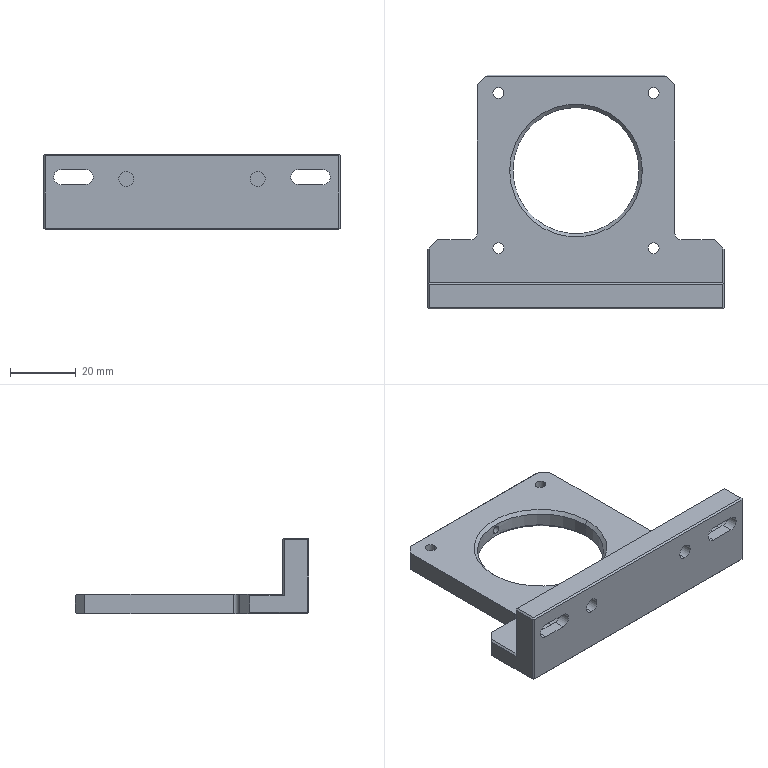Part | NX | features BREP 1 | 1 solid | 75 faces | box 90 x 71 x 23 mm | volume 32601 mm3 | plane 45 | cylinder 26 | cone 4 | commonest cylinder face diameters 3.3 x8 4.5 x8 8 x4 2.5 x2 4 x2 38.3 x2